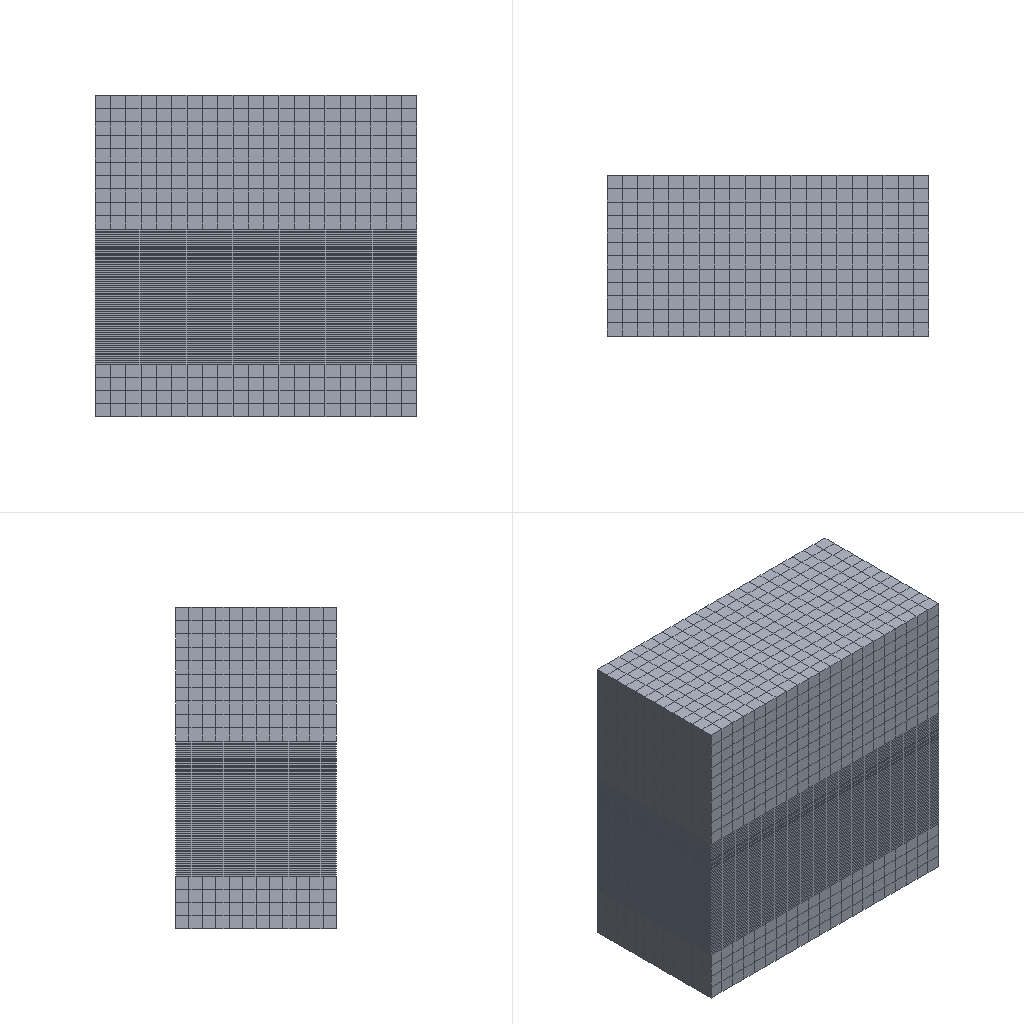Simulation study | abaqus
Set-up summary:
category,name,step,type,value,unit,region
solver,abaqus
solver,version,,,Abaqus/Standard 2020
units,not stated in the deck,,not stated
analysis,deck,,transient,transient
load_step,Step-1,Step-1,transient
load_step,Step-2,Step-2,transient
load_step,requested,,,2
mesh,nodes,,,26210
mesh,elements,,,22895
element_type,C3D8,,solid,22428
element_type,R3D4,,rigid,467
load,load commands in deck,,count,1
bc,support commands in deck,,count,13
material,CR,,in results
material,CRN,,in results
material,DLC,,in results
material,YG6,,in results
check,setup vs results,,match,"per instance, exact: element labels, types and connectivity; labels of the nodes the elements use; coordinates of those nodes at SINGLE_PRECISION in 2 of 2 instance(s)"
Abaqus input file, long lists of numbers shortened:
*Heading
** Job name:  Model name: Model-1-group10
** Generated by: Abaqus/CAE 2020
*Preprint, echo=NO, model=NO, history=NO, contact=NO
**
** PARTS
**
*Part, name=work
*Node
      1, 0.0012,           0., 0.000196
      2, 0.0012, -0.0006, 0.000196
** (25738 more lines like these left out)
*Element, type=C3D8
   1,   396,  5197, 22441,  5077,     1,   301,  5011,   328
   2,  5197,  5198, 22442, 22441,   301,   302,  5012,  5011
** (22426 more lines like these left out)
*Nset, nset=Set-13
   293,   294,   295,   296,   297,   298,   299,   300,  4851,  4852,  4853,  4854,  4855,  4856,  4857,  4858
  4859,  4860,  4861,  4862,  4863,  4864,  4865,  4866,  4867,  4868,  4869,  4870,  4871,  4872,  4873,  4874
** (195 more lines like these left out)
*Elset, elset=Set-13, generate
 19909,  22428,      1
*Nset, nset=Set-14
     9,    10,    11,    12,    13,    14,    15,    16,    17,    18,    19,    20,    21,    22,    23,    24
    25,    26,    27,    28,    29,    30,    31,    32,    33,    34,    35,    36,    37,    38,    39,    40
** (1303 more lines like these left out)
*Elset, elset=Set-14
  1261,  1262,  1263,  1264,  1265,  1266,  1267,  1268,  1269,  1270,  1271,  1272,  1273,  1274,  1275,  1276
  1277,  1278,  1279,  1280,  1281,  1282,  1283,  1284,  1285,  1286,  1287,  1288,  1289,  1290,  1291,  1292
** (581 more lines like these left out)
*Nset, nset=Set-15
     1,     2,     3,     4,     5,     6,     7,     8,   301,   302,   303,   304,   305,   306,   307,   308
   309,   310,   311,   312,   313,   314,   315,   316,   317,   318,   319,   320,   321,   322,   323,   324
** (88 more lines like these left out)
*Elset, elset=Set-15, generate
    1,  1008,     1
*Nset, nset=Set-16
     1,     2,     5,     8,     9,    10,    11,    12,    13,    14,    15,    16,    17,    18,    19,    20
    21,    22,    23,    24,    25,    26,    27,    28,    29,    30,    31,    32,    33,    34,    35,    36
** (1321 more lines like these left out)
*Elset, elset=Set-16
  1009,  1010,  1011,  1012,  1013,  1014,  1015,  1016,  1017,  1018,  1019,  1020,  1021,  1022,  1023,  1024
  1025,  1026,  1027,  1028,  1029,  1030,  1031,  1032,  1033,  1034,  1035,  1036,  1037,  1038,  1039,  1040
** (597 more lines like these left out)
** Section: yg6
*Solid Section, elset=Set-15, material=yg6
,
** Section: crN
*Solid Section, elset=Set-16, material=crN
,
** Section: cr
*Solid Section, elset=Set-14, material=cr
,
** Section: dlc
*Solid Section, elset=Set-13, material=DLC
,
*End Part
**
*Part, name=zhui
*Node
      1, 0.0003, -0.0005196,           0.
      2,           0.,           0.,           0.
** (467 more lines like these left out)
*Element, type=R3D4
 1, 120,  95,  40,  41
 2,  39,  40,  95,  97
** (465 more lines like these left out)
*Node
    470, 5.29395592e-20, -0.0003464, 9.20947787e-05
*Nset, nset=zhui-RefPt_, internal
470,
*Elset, elset=zhui, generate
   1,  467,    1
*End Part
**
**
** ASSEMBLY
**
*Assembly, name=Assembly
**
*Instance, name=work-1, part=work
*End Instance
**
*Instance, name=zhui-1, part=zhui
      0.0006, -5.39999999999999e-05,     0.001292
      0.0006, -5.39999999999999e-05,     0.001292,       0.0006,     0.9999,     0.001292,         180.
*End Instance
**
*Nset, nset=Set-1, instance=work-1
    3,    4,    6,    7,  315,  316,  317,  318,  319,  320,  321,  322,  323,  324,  325,  343
  344,  345,  346,  347,  348,  349,  350,  351,  352,  353,  357,  358,  359,  360,  361,  362
** (16 more lines like these left out)
*Elset, elset=Set-1, instance=work-1
   37,   38,   39,   40,   41,   42,   43,   44,   45,   46,   47,   48,   85,   86,   87,   88
   89,   90,   91,   92,   93,   94,   95,   96,  133,  134,  135,  136,  137,  138,  139,  140
** (14 more lines like these left out)
*Nset, nset=Set-2, instance=zhui-1
 470,
*Nset, nset=Set-3, instance=zhui-1
 470,
*Elset, elset=_m_Surf-1_SPOS, internal, instance=zhui-1, generate
   1,  248,    1
*Surface, type=ELEMENT, name=m_Surf-1
_m_Surf-1_SPOS, SPOS
*Elset, elset=_s_Surf-1_S5, internal, instance=work-1
 20017, 20018, 20019, 20020, 20021, 20022, 20023, 20024, 20025, 20026, 20027, 20028, 20137, 20138, 20139, 20140
 20141, 20142, 20143, 20144, 20145, 20146, 20147, 20148, 20257, 20258, 20259, 20260, 20261, 20262, 20263, 20264
** (14 more lines like these left out)
*Surface, type=ELEMENT, name=s_Surf-1
_s_Surf-1_S5, S5
*Rigid Body, ref node=zhui-1.zhui-RefPt_, elset=zhui-1.zhui
*End Assembly
**
** MATERIALS
**
*Material, name=DLC
*Density
 4e-09,
*Elastic
258800., 0.3
*Material, name=cr
*Density
 7.19e-09,
*Elastic
275000., 0.21
*Plastic
2000.,  0.
5000., 0.1
5500.,  1.
*Material, name=crN
*Density
 5.9e-09,
*Elastic
490000., 0.21
*Plastic
10000.,   0.
15000., 0.01
25000., 0.05
*Material, name=yg6
*Density
 1.5e-08,
*Elastic
71000., 0.3
*Plastic
3000.,0.
**
** INTERACTION PROPERTIES
**
*Surface Interaction, name=IntProp-1
1.,
*Friction, slip tolerance=0.005
 0.3,
*Surface Behavior, pressure-overclosure=HARD
**
** BOUNDARY CONDITIONS
**
** Name: BC-1 Type: 对称/反对称/完全固定
*Boundary
Set-1, ENCASTRE
**
** INTERACTIONS
**
** Interaction: Int-1
*Contact Pair, interaction=IntProp-1, type=SURFACE TO SURFACE
s_Surf-1, m_Surf-1
** Interaction: Int-2
*Contact
*Contact Inclusions, ALL EXTERIOR
*Contact Property Assignment
 ,  , IntProp-1
** ----------------------------------------------------------------
**
** STEP: Step-1
**
*Step, name=Step-1, nlgeom=YES, inc=10000
*Dynamic
0.001,10.,0.0001
**
** BOUNDARY CONDITIONS
**
** Name: BC-2 Type: 位移/转角
*Boundary
Set-2, 1, 1
Set-2, 2, 2
Set-2, 3, 3, -5e-05
Set-2, 4, 4
Set-2, 5, 5
Set-2, 6, 6
**
** OUTPUT REQUESTS
**
*Restart, write, frequency=0
**
** FIELD OUTPUT: F-Output-1
**
*Output, field, frequency=1
*Node Output
A, CF, RF, U, V
*Element Output, directions=YES
E, LE, MISES, PE, PEEQ, PEMAG, S
*Contact Output
CDISP, CSTRESS
**
** HISTORY OUTPUT: H-Output-1
**
*Output, history, variable=PRESELECT
*End Step
** ----------------------------------------------------------------
**
** STEP: Step-2
**
*Step, name=Step-2, nlgeom=YES, inc=1000
*Dynamic
0.01,1.,1e-05
**
** BOUNDARY CONDITIONS
**
** Name: BC-1 Type: 对称/反对称/完全固定
*Boundary, op=NEW
Set-1, ENCASTRE
** Name: BC-2 Type: 位移/转角
*Boundary, op=NEW
Set-2, 1, 1
Set-2, 2, 2
Set-2, 4, 4
Set-2, 5, 5
Set-2, 6, 6
**
** OUTPUT REQUESTS
**
*Restart, write, frequency=0
**
** FIELD OUTPUT: F-Output-1
**
*Output, field, frequency=1
*Node Output
A, CF, RF, U, V
*Element Output, directions=YES
E, LE, MISES, PE, PEEQ, PEMAG, S
*Contact Output
CDISP, CSTRESS
**
** HISTORY OUTPUT: H-Output-1
**
*Output, history, variable=PRESELECT
*End Step
Results summary:
result,step,,completed,increments=27 time=10.0/10.0
result,step,,partial,increments=8 time=0.01803/1.0
result,analysis,,,transient
result,last_loadstep,,,2
result,primary field,,,U
result,reaction total,,FX,-0.0,model units
result,reaction total,,FY,2.9e-05,model units
result,reaction total,,FZ,-3.9e-05,model units